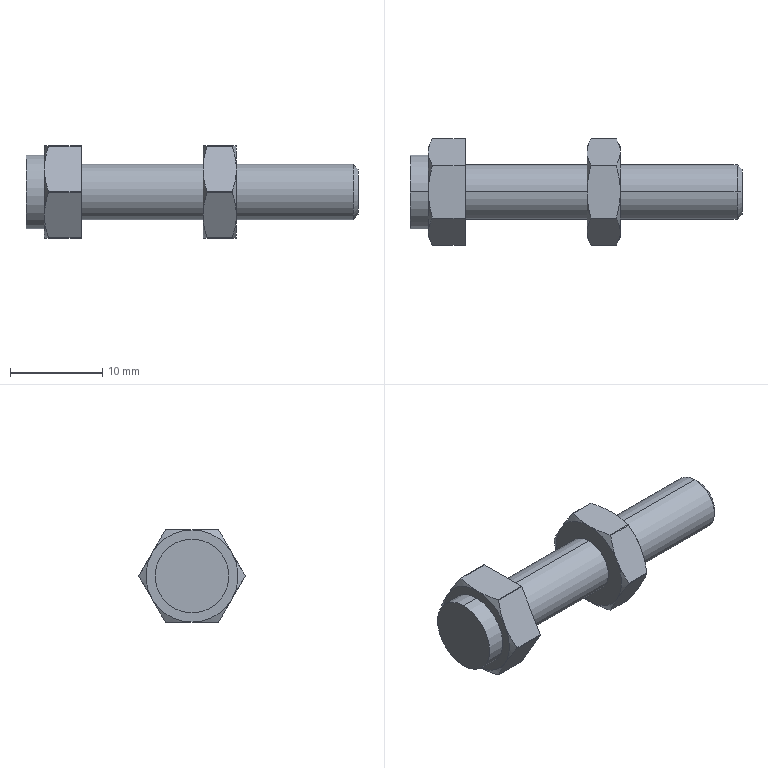Part | STEP file | Mount electronic clip sUSTH6-30 | 2 solids | 67 faces | box 36 x 11.5 x 10 mm | volume 1504 mm3 | plane 25 | cone 24 | cylinder 18 | commonest cylinder face diameters 11.5 x12 4.917 x2 6 x2 8 x2